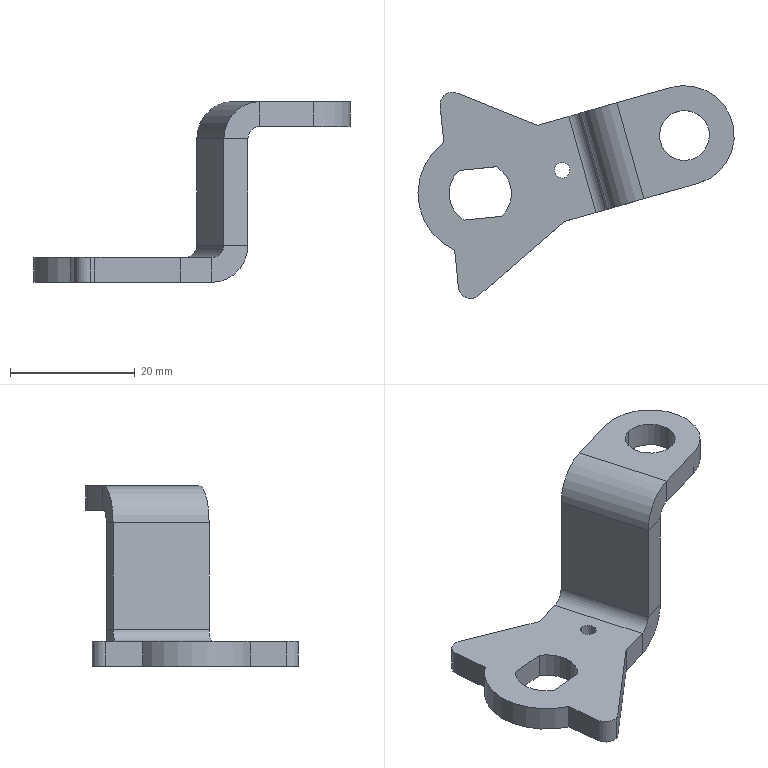Part | SolidWorks | features BaseBody 1 | 1 solid | 37 faces | box 50.722 x 34.063 x 29 mm | volume 4668 mm3 | plane 22 | cylinder 15 | commonest cylinder face diameters 4 x5 2.5 x2 8 x2 10 x2 12 x2 16 x1
STEP:
#1=CARTESIAN_POINT('',(438.908,43.386,86.7));
#2=VERTEX_POINT('',#1);
#3=CARTESIAN_POINT('',(436.735,51.085,86.7));
#4=VERTEX_POINT('',#3);
#5=CARTESIAN_POINT('',(437.822,47.235,86.7));
#6=DIRECTION('',(0.,0.,1.));
#7=DIRECTION('',(-0.2716,0.9624,0.));
#8=AXIS2_PLACEMENT_3D('',#5,#6,#7);
#9=CIRCLE('',#8,4.);
#10=EDGE_CURVE('',#2,#4,#9,.T.);
#11=ORIENTED_EDGE('',*,*,#10,.T.);
#12=CARTESIAN_POINT('',(436.735,51.085,82.7));
#13=VERTEX_POINT('',#12);
#14=CARTESIAN_POINT('',(436.735,51.085,86.7));
#15=DIRECTION('',(0.,0.,-1.));
#16=VECTOR('',#15,1000.);
#17=LINE('',#14,#16);
#18=EDGE_CURVE('',#4,#13,#17,.T.);
#19=ORIENTED_EDGE('',*,*,#18,.T.);
#20=CARTESIAN_POINT('',(438.908,43.386,82.7));
#21=VERTEX_POINT('',#20);
#22=CARTESIAN_POINT('',(437.822,47.235,82.7));
#23=DIRECTION('',(0.,0.,1.));
#24=DIRECTION('',(-0.2716,0.9624,0.));
#25=AXIS2_PLACEMENT_3D('',#22,#23,#24);
#26=CIRCLE('',#25,4.);
#27=EDGE_CURVE('',#21,#13,#26,.T.);
#28=ORIENTED_EDGE('',*,*,#27,.F.);
#29=CARTESIAN_POINT('',(438.908,43.386,86.7));
#30=DIRECTION('',(0.,0.,-1.));
#31=VECTOR('',#30,1000.);
#32=LINE('',#29,#31);
#33=EDGE_CURVE('',#2,#21,#32,.T.);
#34=ORIENTED_EDGE('',*,*,#33,.F.);
#35=EDGE_LOOP('',(#11,#19,#28,#34));
#36=FACE_OUTER_BOUND('',#35,.T.);
#37=CARTESIAN_POINT('',(437.822,47.235,86.7));
#38=DIRECTION('',(0.,0.,-1.));
#39=DIRECTION('',(0.2716,-0.9624,0.));
#40=AXIS2_PLACEMENT_3D('',#37,#38,#39);
#41=CYLINDRICAL_SURFACE('',#40,4.);
#42=ADVANCED_FACE('',(#36),#41,.F.);
#43=CARTESIAN_POINT('',(404.124,21.248,61.7));
#44=VERTEX_POINT('',#43);
#45=CARTESIAN_POINT('',(404.887,21.658,61.7));
#46=VERTEX_POINT('',#45);
#47=CARTESIAN_POINT('',(403.581,23.173,61.7));
#48=DIRECTION('',(0.,0.,1.));
#49=DIRECTION('',(0.2716,-0.9624,0.));
#50=AXIS2_PLACEMENT_3D('',#47,#48,#49);
#51=CIRCLE('',#50,2.);
#52=EDGE_CURVE('',#44,#46,#51,.T.);
#53=ORIENTED_EDGE('',*,*,#52,.F.);
#54=CARTESIAN_POINT('',(404.124,21.248,57.7));
#55=VERTEX_POINT('',#54);
#56=CARTESIAN_POINT('',(404.124,21.248,61.7));
#57=DIRECTION('',(0.,0.,-1.));
#58=VECTOR('',#57,1000.);
#59=LINE('',#56,#58);
#60=EDGE_CURVE('',#44,#55,#59,.T.);
#61=ORIENTED_EDGE('',*,*,#60,.T.);
#62=CARTESIAN_POINT('',(404.887,21.658,57.7));
#63=VERTEX_POINT('',#62);
#64=CARTESIAN_POINT('',(403.581,23.173,57.7));
#65=DIRECTION('',(0.,0.,1.));
#66=DIRECTION('',(0.2716,-0.9624,0.));
#67=AXIS2_PLACEMENT_3D('',#64,#65,#66);
#68=CIRCLE('',#67,2.);
#69=EDGE_CURVE('',#55,#63,#68,.T.);
#70=ORIENTED_EDGE('',*,*,#69,.T.);
#71=CARTESIAN_POINT('',(404.887,21.658,61.7));
#72=DIRECTION('',(0.,0.,-1.));
#73=VECTOR('',#72,1000.);
#74=LINE('',#71,#73);
#75=EDGE_CURVE('',#46,#63,#74,.T.);
#76=ORIENTED_EDGE('',*,*,#75,.F.);
#77=EDGE_LOOP('',(#53,#61,#70,#76));
#78=FACE_OUTER_BOUND('',#77,.T.);
#79=CARTESIAN_POINT('',(403.581,23.173,61.7));
#80=DIRECTION('',(0.,0.,-1.));
#81=DIRECTION('',(0.2716,-0.9624,0.));
#82=AXIS2_PLACEMENT_3D('',#79,#80,#81);
#83=CYLINDRICAL_SURFACE('',#82,2.);
#84=ADVANCED_FACE('',(#78),#83,.T.);
#85=CARTESIAN_POINT('',(418.576,40.505,61.7));
#86=VERTEX_POINT('',#85);
#87=CARTESIAN_POINT('',(417.897,42.911,61.7));
#88=VERTEX_POINT('',#87);
#89=CARTESIAN_POINT('',(418.237,41.708,61.7));
#90=DIRECTION('',(0.,0.,1.));
#91=DIRECTION('',(-0.2716,0.9624,0.));
#92=AXIS2_PLACEMENT_3D('',#89,#90,#91);
#93=CIRCLE('',#92,1.25);
#94=EDGE_CURVE('',#86,#88,#93,.T.);
#95=ORIENTED_EDGE('',*,*,#94,.T.);
#96=CARTESIAN_POINT('',(417.897,42.911,57.7));
#97=VERTEX_POINT('',#96);
#98=CARTESIAN_POINT('',(417.897,42.911,61.7));
#99=DIRECTION('',(0.,0.,-1.));
#100=VECTOR('',#99,1000.);
#101=LINE('',#98,#100);
#102=EDGE_CURVE('',#88,#97,#101,.T.);
#103=ORIENTED_EDGE('',*,*,#102,.T.);
#104=CARTESIAN_POINT('',(418.576,40.505,57.7));
#105=VERTEX_POINT('',#104);
#106=CARTESIAN_POINT('',(418.237,41.708,57.7));
#107=DIRECTION('',(0.,0.,1.));
#108=DIRECTION('',(-0.2716,0.9624,0.));
#109=AXIS2_PLACEMENT_3D('',#106,#107,#108);
#110=CIRCLE('',#109,1.25);
#111=EDGE_CURVE('',#105,#97,#110,.T.);
#112=ORIENTED_EDGE('',*,*,#111,.F.);
#113=CARTESIAN_POINT('',(418.576,40.505,61.7));
#114=DIRECTION('',(0.,0.,-1.));
#115=VECTOR('',#114,1000.);
#116=LINE('',#113,#115);
#117=EDGE_CURVE('',#86,#105,#116,.T.);
#118=ORIENTED_EDGE('',*,*,#117,.F.);
#119=EDGE_LOOP('',(#95,#103,#112,#118));
#120=FACE_OUTER_BOUND('',#119,.T.);
#121=CARTESIAN_POINT('',(418.237,41.708,61.7));
#122=DIRECTION('',(0.,0.,-1.));
#123=DIRECTION('',(0.2716,-0.9624,0.));
#124=AXIS2_PLACEMENT_3D('',#121,#122,#123);
#125=CYLINDRICAL_SURFACE('',#124,1.25);
#126=ADVANCED_FACE('',(#120),#125,.F.);
#127=CARTESIAN_POINT('',(425.062,51.947,80.7));
#128=VERTEX_POINT('',#127);
#129=CARTESIAN_POINT('',(425.062,51.947,63.7));
#130=VERTEX_POINT('',#129);
#131=CARTESIAN_POINT('',(425.062,51.947,52.207));
#132=DIRECTION('',(0.,0.,-1.));
#133=VECTOR('',#132,1000.);
#134=LINE('',#131,#133);
#135=EDGE_CURVE('',#128,#130,#134,.T.);
#136=ORIENTED_EDGE('',*,*,#135,.F.);
#137=CARTESIAN_POINT('',(429.408,36.548,80.7));
#138=VERTEX_POINT('',#137);
#139=CARTESIAN_POINT('',(427.235,44.248,80.7));
#140=DIRECTION('',(0.2716,-0.9624,0.));
#141=VECTOR('',#140,1000.);
#142=LINE('',#139,#141);
#143=EDGE_CURVE('',#128,#138,#142,.T.);
#144=ORIENTED_EDGE('',*,*,#143,.T.);
#145=CARTESIAN_POINT('',(429.408,36.548,63.7));
#146=VERTEX_POINT('',#145);
#147=CARTESIAN_POINT('',(429.408,36.548,52.207));
#148=DIRECTION('',(0.,0.,1.));
#149=VECTOR('',#148,1000.);
#150=LINE('',#147,#149);
#151=EDGE_CURVE('',#146,#138,#150,.T.);
#152=ORIENTED_EDGE('',*,*,#151,.F.);
#153=CARTESIAN_POINT('',(427.235,44.248,63.7));
#154=DIRECTION('',(0.2716,-0.9624,0.));
#155=VECTOR('',#154,1000.);
#156=LINE('',#153,#155);
#157=EDGE_CURVE('',#130,#146,#156,.T.);
#158=ORIENTED_EDGE('',*,*,#157,.F.);
#159=EDGE_LOOP('',(#136,#144,#152,#158));
#160=FACE_OUTER_BOUND('',#159,.T.);
#161=CARTESIAN_POINT('',(427.235,44.248,74.417));
#162=DIRECTION('',(-0.9624,-0.2716,0.));
#163=DIRECTION('',(-0.2716,0.9624,0.));
#164=AXIS2_PLACEMENT_3D('',#161,#162,#163);
#165=PLANE('',#164);
#166=ADVANCED_FACE('',(#160),#165,.F.);
#167=CARTESIAN_POINT('',(421.213,50.86,80.7));
#168=VERTEX_POINT('',#167);
#169=CARTESIAN_POINT('',(421.213,50.86,63.7));
#170=VERTEX_POINT('',#169);
#171=CARTESIAN_POINT('',(421.213,50.86,52.207));
#172=DIRECTION('',(0.,0.,-1.));
#173=VECTOR('',#172,1000.);
#174=LINE('',#171,#173);
#175=EDGE_CURVE('',#168,#170,#174,.T.);
#176=ORIENTED_EDGE('',*,*,#175,.F.);
#177=CARTESIAN_POINT('',(421.213,50.86,80.7));
#178=DIRECTION('',(0.9624,0.2716,0.));
#179=VECTOR('',#178,1000.);
#180=LINE('',#177,#179);
#181=EDGE_CURVE('',#168,#128,#180,.T.);
#182=ORIENTED_EDGE('',*,*,#181,.T.);
#183=ORIENTED_EDGE('',*,*,#135,.T.);
#184=CARTESIAN_POINT('',(421.213,50.86,63.7));
#185=DIRECTION('',(0.9624,0.2716,0.));
#186=VECTOR('',#185,1000.);
#187=LINE('',#184,#186);
#188=EDGE_CURVE('',#170,#130,#187,.T.);
#189=ORIENTED_EDGE('',*,*,#188,.F.);
#190=EDGE_LOOP('',(#176,#182,#183,#189));
#191=FACE_OUTER_BOUND('',#190,.T.);
#192=CARTESIAN_POINT('',(421.213,50.86,52.207));
#193=DIRECTION('',(0.2716,-0.9624,0.));
#194=DIRECTION('',(0.,0.,1.));
#195=AXIS2_PLACEMENT_3D('',#192,#193,#194);
#196=PLANE('',#195);
#197=ADVANCED_FACE('',(#191),#196,.F.);
#198=ORIENTED_EDGE('',*,*,#151,.T.);
#199=CARTESIAN_POINT('',(425.559,35.462,80.7));
#200=VERTEX_POINT('',#199);
#201=CARTESIAN_POINT('',(425.559,35.462,80.7));
#202=DIRECTION('',(-0.9624,-0.2716,0.));
#203=VECTOR('',#202,1000.);
#204=LINE('',#201,#203);
#205=EDGE_CURVE('',#138,#200,#204,.T.);
#206=ORIENTED_EDGE('',*,*,#205,.T.);
#207=CARTESIAN_POINT('',(425.559,35.462,63.7));
#208=VERTEX_POINT('',#207);
#209=CARTESIAN_POINT('',(425.559,35.462,52.207));
#210=DIRECTION('',(0.,0.,1.));
#211=VECTOR('',#210,1000.);
#212=LINE('',#209,#211);
#213=EDGE_CURVE('',#208,#200,#212,.T.);
#214=ORIENTED_EDGE('',*,*,#213,.F.);
#215=CARTESIAN_POINT('',(425.559,35.462,63.7));
#216=DIRECTION('',(-0.9624,-0.2716,0.));
#217=VECTOR('',#216,1000.);
#218=LINE('',#215,#217);
#219=EDGE_CURVE('',#146,#208,#218,.T.);
#220=ORIENTED_EDGE('',*,*,#219,.F.);
#221=EDGE_LOOP('',(#198,#206,#214,#220));
#222=FACE_OUTER_BOUND('',#221,.T.);
#223=CARTESIAN_POINT('',(425.559,35.462,52.207));
#224=DIRECTION('',(-0.2716,0.9624,0.));
#225=DIRECTION('',(0.,0.,-1.));
#226=AXIS2_PLACEMENT_3D('',#223,#224,#225);
#227=PLANE('',#226);
#228=ADVANCED_FACE('',(#222),#227,.F.);
#229=CARTESIAN_POINT('',(423.386,43.161,80.7));
#230=DIRECTION('',(0.2716,-0.9624,0.));
#231=VECTOR('',#230,1000.);
#232=LINE('',#229,#231);
#233=EDGE_CURVE('',#168,#200,#232,.T.);
#234=ORIENTED_EDGE('',*,*,#233,.F.);
#235=ORIENTED_EDGE('',*,*,#175,.T.);
#236=CARTESIAN_POINT('',(423.386,43.161,63.7));
#237=DIRECTION('',(0.2716,-0.9624,0.));
#238=VECTOR('',#237,1000.);
#239=LINE('',#236,#238);
#240=EDGE_CURVE('',#170,#208,#239,.T.);
#241=ORIENTED_EDGE('',*,*,#240,.T.);
#242=ORIENTED_EDGE('',*,*,#213,.T.);
#243=EDGE_LOOP('',(#234,#235,#241,#242));
#244=FACE_OUTER_BOUND('',#243,.T.);
#245=CARTESIAN_POINT('',(423.386,43.161,74.417));
#246=DIRECTION('',(-0.9624,-0.2716,0.));
#247=DIRECTION('',(-0.2716,0.9624,0.));
#248=AXIS2_PLACEMENT_3D('',#245,#246,#247);
#249=PLANE('',#248);
#250=ADVANCED_FACE('',(#244),#249,.T.);
#251=ORIENTED_EDGE('',*,*,#102,.F.);
#252=CARTESIAN_POINT('',(418.237,41.708,61.7));
#253=DIRECTION('',(0.,0.,1.));
#254=DIRECTION('',(-0.2716,0.9624,0.));
#255=AXIS2_PLACEMENT_3D('',#252,#253,#254);
#256=CIRCLE('',#255,1.25);
#257=EDGE_CURVE('',#88,#86,#256,.T.);
#258=ORIENTED_EDGE('',*,*,#257,.T.);
#259=ORIENTED_EDGE('',*,*,#117,.T.);
#260=CARTESIAN_POINT('',(418.237,41.708,57.7));
#261=DIRECTION('',(0.,0.,1.));
#262=DIRECTION('',(-0.2716,0.9624,0.));
#263=AXIS2_PLACEMENT_3D('',#260,#261,#262);
#264=CIRCLE('',#263,1.25);
#265=EDGE_CURVE('',#97,#105,#264,.T.);
#266=ORIENTED_EDGE('',*,*,#265,.F.);
#267=EDGE_LOOP('',(#251,#258,#259,#266));
#268=FACE_OUTER_BOUND('',#267,.T.);
#269=CARTESIAN_POINT('',(418.237,41.708,61.7));
#270=DIRECTION('',(0.,0.,-1.));
#271=DIRECTION('',(0.2716,-0.9624,0.));
#272=AXIS2_PLACEMENT_3D('',#269,#270,#271);
#273=CYLINDRICAL_SURFACE('',#272,1.25);
#274=ADVANCED_FACE('',(#268),#273,.F.);
#275=CARTESIAN_POINT('',(408.486,34.321,57.7));
#276=VERTEX_POINT('',#275);
#277=CARTESIAN_POINT('',(407.683,42.281,57.7));
#278=VERTEX_POINT('',#277);
#279=CARTESIAN_POINT('',(405.1,38.,57.7));
#280=DIRECTION('',(0.,0.,1.));
#281=DIRECTION('',(-0.2716,0.9624,0.));
#282=AXIS2_PLACEMENT_3D('',#279,#280,#281);
#283=CIRCLE('',#282,5.);
#284=EDGE_CURVE('',#276,#278,#283,.T.);
#285=ORIENTED_EDGE('',*,*,#284,.F.);
#286=CARTESIAN_POINT('',(408.486,34.321,61.7));
#287=VERTEX_POINT('',#286);
#288=CARTESIAN_POINT('',(408.486,34.321,61.7));
#289=DIRECTION('',(0.,0.,-1.));
#290=VECTOR('',#289,1000.);
#291=LINE('',#288,#290);
#292=EDGE_CURVE('',#287,#276,#291,.T.);
#293=ORIENTED_EDGE('',*,*,#292,.F.);
#294=CARTESIAN_POINT('',(407.683,42.281,61.7));
#295=VERTEX_POINT('',#294);
#296=CARTESIAN_POINT('',(405.1,38.,61.7));
#297=DIRECTION('',(0.,0.,1.));
#298=DIRECTION('',(-0.2716,0.9624,0.));
#299=AXIS2_PLACEMENT_3D('',#296,#297,#298);
#300=CIRCLE('',#299,5.);
#301=EDGE_CURVE('',#287,#295,#300,.T.);
#302=ORIENTED_EDGE('',*,*,#301,.T.);
#303=CARTESIAN_POINT('',(407.683,42.281,61.7));
#304=DIRECTION('',(0.,0.,-1.));
#305=VECTOR('',#304,1000.);
#306=LINE('',#303,#305);
#307=EDGE_CURVE('',#295,#278,#306,.T.);
#308=ORIENTED_EDGE('',*,*,#307,.T.);
#309=EDGE_LOOP('',(#285,#293,#302,#308));
#310=FACE_OUTER_BOUND('',#309,.T.);
#311=CARTESIAN_POINT('',(405.1,38.,61.7));
#312=DIRECTION('',(0.,0.,-1.));
#313=DIRECTION('',(0.2716,-0.9624,0.));
#314=AXIS2_PLACEMENT_3D('',#311,#312,#313);
#315=CYLINDRICAL_SURFACE('',#314,5.);
#316=ADVANCED_FACE('',(#310),#315,.F.);
#317=CARTESIAN_POINT('',(401.714,41.679,57.7));
#318=VERTEX_POINT('',#317);
#319=CARTESIAN_POINT('',(401.714,41.679,57.7));
#320=DIRECTION('',(-0.9949,-0.1004,0.));
#321=VECTOR('',#320,1000.);
#322=LINE('',#319,#321);
#323=EDGE_CURVE('',#278,#318,#322,.T.);
#324=ORIENTED_EDGE('',*,*,#323,.F.);
#325=ORIENTED_EDGE('',*,*,#307,.F.);
#326=CARTESIAN_POINT('',(401.714,41.679,61.7));
#327=VERTEX_POINT('',#326);
#328=CARTESIAN_POINT('',(401.714,41.679,61.7));
#329=DIRECTION('',(-0.9949,-0.1004,0.));
#330=VECTOR('',#329,1000.);
#331=LINE('',#328,#330);
#332=EDGE_CURVE('',#295,#327,#331,.T.);
#333=ORIENTED_EDGE('',*,*,#332,.T.);
#334=CARTESIAN_POINT('',(401.714,41.679,61.7));
#335=DIRECTION('',(0.,0.,-1.));
#336=VECTOR('',#335,1000.);
#337=LINE('',#334,#336);
#338=EDGE_CURVE('',#327,#318,#337,.T.);
#339=ORIENTED_EDGE('',*,*,#338,.T.);
#340=EDGE_LOOP('',(#324,#325,#333,#339));
#341=FACE_OUTER_BOUND('',#340,.T.);
#342=CARTESIAN_POINT('',(401.714,41.679,61.7));
#343=DIRECTION('',(0.1004,-0.9949,0.));
#344=DIRECTION('',(0.9949,0.1004,0.));
#345=AXIS2_PLACEMENT_3D('',#342,#343,#344);
#346=PLANE('',#345);
#347=ADVANCED_FACE('',(#341),#346,.T.);
#348=CARTESIAN_POINT('',(402.517,33.719,57.7));
#349=VERTEX_POINT('',#348);
#350=CARTESIAN_POINT('',(405.1,38.,57.7));
#351=DIRECTION('',(0.,0.,1.));
#352=DIRECTION('',(-0.2716,0.9624,0.));
#353=AXIS2_PLACEMENT_3D('',#350,#351,#352);
#354=CIRCLE('',#353,5.);
#355=EDGE_CURVE('',#318,#349,#354,.T.);
#356=ORIENTED_EDGE('',*,*,#355,.F.);
#357=ORIENTED_EDGE('',*,*,#338,.F.);
#358=CARTESIAN_POINT('',(402.517,33.719,61.7));
#359=VERTEX_POINT('',#358);
#360=CARTESIAN_POINT('',(405.1,38.,61.7));
#361=DIRECTION('',(0.,0.,1.));
#362=DIRECTION('',(-0.2716,0.9624,0.));
#363=AXIS2_PLACEMENT_3D('',#360,#361,#362);
#364=CIRCLE('',#363,5.);
#365=EDGE_CURVE('',#327,#359,#364,.T.);
#366=ORIENTED_EDGE('',*,*,#365,.T.);
#367=CARTESIAN_POINT('',(402.517,33.719,61.7));
#368=DIRECTION('',(0.,0.,-1.));
#369=VECTOR('',#368,1000.);
#370=LINE('',#367,#369);
#371=EDGE_CURVE('',#359,#349,#370,.T.);
#372=ORIENTED_EDGE('',*,*,#371,.T.);
#373=EDGE_LOOP('',(#356,#357,#366,#372));
#374=FACE_OUTER_BOUND('',#373,.T.);
#375=CARTESIAN_POINT('',(405.1,38.,61.7));
#376=DIRECTION('',(0.,0.,-1.));
#377=DIRECTION('',(0.2716,-0.9624,0.));
#378=AXIS2_PLACEMENT_3D('',#375,#376,#377);
#379=CYLINDRICAL_SURFACE('',#378,5.);
#380=ADVANCED_FACE('',(#374),#379,.F.);
#381=CARTESIAN_POINT('',(402.517,33.719,57.7));
#382=DIRECTION('',(0.9949,0.1004,0.));
#383=VECTOR('',#382,1000.);
#384=LINE('',#381,#383);
#385=EDGE_CURVE('',#349,#276,#384,.T.);
#386=ORIENTED_EDGE('',*,*,#385,.F.);
#387=ORIENTED_EDGE('',*,*,#371,.F.);
#388=CARTESIAN_POINT('',(402.517,33.719,61.7));
#389=DIRECTION('',(0.9949,0.1004,0.));
#390=VECTOR('',#389,1000.);
#391=LINE('',#388,#390);
#392=EDGE_CURVE('',#359,#287,#391,.T.);
#393=ORIENTED_EDGE('',*,*,#392,.T.);
#394=ORIENTED_EDGE('',*,*,#292,.T.);
#395=EDGE_LOOP('',(#386,#387,#393,#394));
#396=FACE_OUTER_BOUND('',#395,.T.);
#397=CARTESIAN_POINT('',(402.517,33.719,61.7));
#398=DIRECTION('',(-0.1004,0.9949,0.));
#399=DIRECTION('',(-0.9949,-0.1004,0.));
#400=AXIS2_PLACEMENT_3D('',#397,#398,#399);
#401=PLANE('',#400);
#402=ADVANCED_FACE('',(#396),#401,.T.);
#403=CARTESIAN_POINT('',(418.62,33.503,57.7));
#404=VERTEX_POINT('',#403);
#405=CARTESIAN_POINT('',(418.62,33.503,57.7));
#406=DIRECTION('',(0.7572,0.6532,0.));
#407=VECTOR('',#406,1000.);
#408=LINE('',#405,#407);
#409=EDGE_CURVE('',#63,#404,#408,.T.);
#410=ORIENTED_EDGE('',*,*,#409,.T.);
#411=CARTESIAN_POINT('',(418.62,33.503,61.7));
#412=VERTEX_POINT('',#411);
#413=CARTESIAN_POINT('',(418.62,33.503,61.7));
#414=DIRECTION('',(0.,0.,-1.));
#415=VECTOR('',#414,1000.);
#416=LINE('',#413,#415);
#417=EDGE_CURVE('',#412,#404,#416,.T.);
#418=ORIENTED_EDGE('',*,*,#417,.F.);
#419=CARTESIAN_POINT('',(418.62,33.503,61.7));
#420=DIRECTION('',(0.7572,0.6532,0.));
#421=VECTOR('',#420,1000.);
#422=LINE('',#419,#421);
#423=EDGE_CURVE('',#46,#412,#422,.T.);
#424=ORIENTED_EDGE('',*,*,#423,.F.);
#425=ORIENTED_EDGE('',*,*,#75,.T.);
#426=EDGE_LOOP('',(#410,#418,#424,#425));
#427=FACE_OUTER_BOUND('',#426,.T.);
#428=CARTESIAN_POINT('',(418.62,33.503,61.7));
#429=DIRECTION('',(-0.6532,0.7572,0.));
#430=DIRECTION('',(-0.7572,-0.6532,0.));
#431=AXIS2_PLACEMENT_3D('',#428,#429,#430);
#432=PLANE('',#431);
#433=ADVANCED_FACE('',(#427),#432,.F.);
#434=ORIENTED_EDGE('',*,*,#60,.F.);
#435=CARTESIAN_POINT('',(401.591,22.972,61.7));
#436=VERTEX_POINT('',#435);
#437=CARTESIAN_POINT('',(403.581,23.173,61.7));
#438=DIRECTION('',(0.,0.,1.));
#439=DIRECTION('',(0.2716,-0.9624,0.));
#440=AXIS2_PLACEMENT_3D('',#437,#438,#439);
#441=CIRCLE('',#440,2.);
#442=EDGE_CURVE('',#436,#44,#441,.T.);
#443=ORIENTED_EDGE('',*,*,#442,.F.);
#444=CARTESIAN_POINT('',(401.591,22.972,57.7));
#445=VERTEX_POINT('',#444);
#446=CARTESIAN_POINT('',(401.591,22.972,61.7));
#447=DIRECTION('',(0.,0.,-1.));
#448=VECTOR('',#447,1000.);
#449=LINE('',#446,#448);
#450=EDGE_CURVE('',#436,#445,#449,.T.);
#451=ORIENTED_EDGE('',*,*,#450,.T.);
#452=CARTESIAN_POINT('',(403.581,23.173,57.7));
#453=DIRECTION('',(0.,0.,1.));
#454=DIRECTION('',(0.2716,-0.9624,0.));
#455=AXIS2_PLACEMENT_3D('',#452,#453,#454);
#456=CIRCLE('',#455,2.);
#457=EDGE_CURVE('',#445,#55,#456,.T.);
#458=ORIENTED_EDGE('',*,*,#457,.T.);
#459=EDGE_LOOP('',(#434,#443,#451,#458));
#460=FACE_OUTER_BOUND('',#459,.T.);
#461=CARTESIAN_POINT('',(403.581,23.173,61.7));
#462=DIRECTION('',(0.,0.,-1.));
#463=DIRECTION('',(0.2716,-0.9624,0.));
#464=AXIS2_PLACEMENT_3D('',#461,#462,#463);
#465=CYLINDRICAL_SURFACE('',#464,2.);
#466=ADVANCED_FACE('',(#460),#465,.T.);
#467=CARTESIAN_POINT('',(400.995,28.882,57.7));
#468=VERTEX_POINT('',#467);
#469=CARTESIAN_POINT('',(401.591,22.972,57.7));
#470=DIRECTION('',(0.1004,-0.9949,0.));
#471=VECTOR('',#470,1000.);
#472=LINE('',#469,#471);
#473=EDGE_CURVE('',#468,#445,#472,.T.);
#474=ORIENTED_EDGE('',*,*,#473,.T.);
#475=ORIENTED_EDGE('',*,*,#450,.F.);
#476=CARTESIAN_POINT('',(400.995,28.882,61.7));
#477=VERTEX_POINT('',#476);
#478=CARTESIAN_POINT('',(401.591,22.972,61.7));
#479=DIRECTION('',(0.1004,-0.9949,0.));
#480=VECTOR('',#479,1000.);
#481=LINE('',#478,#480);
#482=EDGE_CURVE('',#477,#436,#481,.T.);
#483=ORIENTED_EDGE('',*,*,#482,.F.);
#484=CARTESIAN_POINT('',(400.995,28.882,61.7));
#485=DIRECTION('',(0.,0.,-1.));
#486=VECTOR('',#485,1000.);
#487=LINE('',#484,#486);
#488=EDGE_CURVE('',#477,#468,#487,.T.);
#489=ORIENTED_EDGE('',*,*,#488,.T.);
#490=EDGE_LOOP('',(#474,#475,#483,#489));
#491=FACE_OUTER_BOUND('',#490,.T.);
#492=CARTESIAN_POINT('',(401.591,22.972,61.7));
#493=DIRECTION('',(0.9949,0.1004,0.));
#494=DIRECTION('',(-0.1004,0.9949,0.));
#495=AXIS2_PLACEMENT_3D('',#492,#493,#494);
#496=PLANE('',#495);
#497=ADVANCED_FACE('',(#491),#496,.F.);
#498=CARTESIAN_POINT('',(399.256,46.115,57.7));
#499=VERTEX_POINT('',#498);
#500=CARTESIAN_POINT('',(405.1,38.,57.7));
#501=DIRECTION('',(0.,0.,1.));
#502=DIRECTION('',(-0.2716,0.9624,0.));
#503=AXIS2_PLACEMENT_3D('',#500,#501,#502);
#504=CIRCLE('',#503,10.);
#505=EDGE_CURVE('',#499,#468,#504,.T.);
#506=ORIENTED_EDGE('',*,*,#505,.T.);
#507=ORIENTED_EDGE('',*,*,#488,.F.);
#508=CARTESIAN_POINT('',(399.256,46.115,61.7));
#509=VERTEX_POINT('',#508);
#510=CARTESIAN_POINT('',(405.1,38.,61.7));
#511=DIRECTION('',(0.,0.,1.));
#512=DIRECTION('',(-0.2716,0.9624,0.));
#513=AXIS2_PLACEMENT_3D('',#510,#511,#512);
#514=CIRCLE('',#513,10.);
#515=EDGE_CURVE('',#509,#477,#514,.T.);
#516=ORIENTED_EDGE('',*,*,#515,.F.);
#517=CARTESIAN_POINT('',(399.256,46.115,61.7));
#518=DIRECTION('',(0.,0.,-1.));
#519=VECTOR('',#518,1000.);
#520=LINE('',#517,#519);
#521=EDGE_CURVE('',#509,#499,#520,.T.);
#522=ORIENTED_EDGE('',*,*,#521,.T.);
#523=EDGE_LOOP('',(#506,#507,#516,#522));
#524=FACE_OUTER_BOUND('',#523,.T.);
#525=CARTESIAN_POINT('',(405.1,38.,61.7));
#526=DIRECTION('',(0.,0.,-1.));
#527=DIRECTION('',(0.2716,-0.9624,0.));
#528=AXIS2_PLACEMENT_3D('',#525,#526,#527);
#529=CYLINDRICAL_SURFACE('',#528,10.);
#530=ADVANCED_FACE('',(#524),#529,.T.);
#531=CARTESIAN_POINT('',(398.66,52.024,57.7));
#532=VERTEX_POINT('',#531);
#533=CARTESIAN_POINT('',(399.256,46.115,57.7));
#534=DIRECTION('',(0.1004,-0.9949,0.));
#535=VECTOR('',#534,1000.);
#536=LINE('',#533,#535);
#537=EDGE_CURVE('',#532,#499,#536,.T.);
#538=ORIENTED_EDGE('',*,*,#537,.T.);
#539=ORIENTED_EDGE('',*,*,#521,.F.);
#540=CARTESIAN_POINT('',(398.66,52.024,61.7));
#541=VERTEX_POINT('',#540);
#542=CARTESIAN_POINT('',(399.256,46.115,61.7));
#543=DIRECTION('',(0.1004,-0.9949,0.));
#544=VECTOR('',#543,1000.);
#545=LINE('',#542,#544);
#546=EDGE_CURVE('',#541,#509,#545,.T.);
#547=ORIENTED_EDGE('',*,*,#546,.F.);
#548=CARTESIAN_POINT('',(398.66,52.024,61.7));
#549=DIRECTION('',(0.,0.,-1.));
#550=VECTOR('',#549,1000.);
#551=LINE('',#548,#550);
#552=EDGE_CURVE('',#541,#532,#551,.T.);
#553=ORIENTED_EDGE('',*,*,#552,.T.);
#554=EDGE_LOOP('',(#538,#539,#547,#553));
#555=FACE_OUTER_BOUND('',#554,.T.);
#556=CARTESIAN_POINT('',(399.256,46.115,61.7));
#557=DIRECTION('',(0.9949,0.1004,0.));
#558=DIRECTION('',(-0.1004,0.9949,0.));
#559=AXIS2_PLACEMENT_3D('',#556,#557,#558);
#560=PLANE('',#559);
#561=ADVANCED_FACE('',(#555),#560,.F.);
#562=CARTESIAN_POINT('',(401.396,54.081,57.7));
#563=VERTEX_POINT('',#562);
#564=CARTESIAN_POINT('',(400.65,52.225,57.7));
#565=DIRECTION('',(0.,0.,1.));
#566=DIRECTION('',(-0.2716,0.9624,0.));
#567=AXIS2_PLACEMENT_3D('',#564,#565,#566);
#568=CIRCLE('',#567,2.);
#569=EDGE_CURVE('',#563,#532,#568,.T.);
#570=ORIENTED_EDGE('',*,*,#569,.T.);
#571=ORIENTED_EDGE('',*,*,#552,.F.);
#572=CARTESIAN_POINT('',(401.396,54.081,61.7));
#573=VERTEX_POINT('',#572);
#574=CARTESIAN_POINT('',(400.65,52.225,61.7));
#575=DIRECTION('',(0.,0.,1.));
#576=DIRECTION('',(-0.2716,0.9624,0.));
#577=AXIS2_PLACEMENT_3D('',#574,#575,#576);
#578=CIRCLE('',#577,2.);
#579=EDGE_CURVE('',#573,#541,#578,.T.);
#580=ORIENTED_EDGE('',*,*,#579,.F.);
#581=CARTESIAN_POINT('',(401.396,54.081,61.7));
#582=DIRECTION('',(0.,0.,-1.));
#583=VECTOR('',#582,1000.);
#584=LINE('',#581,#583);
#585=EDGE_CURVE('',#573,#563,#584,.T.);
#586=ORIENTED_EDGE('',*,*,#585,.T.);
#587=EDGE_LOOP('',(#570,#571,#580,#586));
#588=FACE_OUTER_BOUND('',#587,.T.);
#589=CARTESIAN_POINT('',(400.65,52.225,61.7));
#590=DIRECTION('',(0.,0.,-1.));
#591=DIRECTION('',(0.2716,-0.9624,0.));
#592=AXIS2_PLACEMENT_3D('',#589,#590,#591);
#593=CYLINDRICAL_SURFACE('',#592,2.);
#594=ADVANCED_FACE('',(#588),#593,.T.);
#595=CARTESIAN_POINT('',(414.274,48.902,57.7));
#596=VERTEX_POINT('',#595);
#597=CARTESIAN_POINT('',(414.274,48.902,57.7));
#598=DIRECTION('',(-0.9278,0.3731,0.));
#599=VECTOR('',#598,1000.);
#600=LINE('',#597,#599);
#601=EDGE_CURVE('',#596,#563,#600,.T.);
#602=ORIENTED_EDGE('',*,*,#601,.T.);
#603=ORIENTED_EDGE('',*,*,#585,.F.);
#604=CARTESIAN_POINT('',(414.274,48.902,61.7));
#605=VERTEX_POINT('',#604);
#606=CARTESIAN_POINT('',(414.274,48.902,61.7));
#607=DIRECTION('',(-0.9278,0.3731,0.));
#608=VECTOR('',#607,1000.);
#609=LINE('',#606,#608);
#610=EDGE_CURVE('',#605,#573,#609,.T.);
#611=ORIENTED_EDGE('',*,*,#610,.F.);
#612=CARTESIAN_POINT('',(414.274,48.902,61.7));
#613=DIRECTION('',(0.,0.,-1.));
#614=VECTOR('',#613,1000.);
#615=LINE('',#612,#614);
#616=EDGE_CURVE('',#605,#596,#615,.T.);
#617=ORIENTED_EDGE('',*,*,#616,.T.);
#618=EDGE_LOOP('',(#602,#603,#611,#617));
#619=FACE_OUTER_BOUND('',#618,.T.);
#620=CARTESIAN_POINT('',(414.274,48.902,61.7));
#621=DIRECTION('',(-0.3731,-0.9278,0.));
#622=DIRECTION('',(0.9278,-0.3731,0.));
#623=AXIS2_PLACEMENT_3D('',#620,#621,#622);
#624=PLANE('',#623);
#625=ADVANCED_FACE('',(#619),#624,.F.);
#626=CARTESIAN_POINT('',(419.288,50.317,61.7));
#627=VERTEX_POINT('',#626);
#628=CARTESIAN_POINT('',(423.634,34.919,61.7));
#629=VERTEX_POINT('',#628);
#630=CARTESIAN_POINT('',(421.461,42.618,61.7));
#631=DIRECTION('',(0.2716,-0.9624,0.));
#632=VECTOR('',#631,1000.);
#633=LINE('',#630,#632);
#634=EDGE_CURVE('',#627,#629,#633,.T.);
#635=ORIENTED_EDGE('',*,*,#634,.F.);
#636=CARTESIAN_POINT('',(414.274,48.902,61.7));
#637=DIRECTION('',(-0.9624,-0.2716,0.));
#638=VECTOR('',#637,1000.);
#639=LINE('',#636,#638);
#640=EDGE_CURVE('',#627,#605,#639,.T.);
#641=ORIENTED_EDGE('',*,*,#640,.T.);
#642=ORIENTED_EDGE('',*,*,#610,.T.);
#643=ORIENTED_EDGE('',*,*,#579,.T.);
#644=ORIENTED_EDGE('',*,*,#546,.T.);
#645=ORIENTED_EDGE('',*,*,#515,.T.);
#646=ORIENTED_EDGE('',*,*,#482,.T.);
#647=ORIENTED_EDGE('',*,*,#442,.T.);
#648=ORIENTED_EDGE('',*,*,#52,.T.);
#649=ORIENTED_EDGE('',*,*,#423,.T.);
#650=CARTESIAN_POINT('',(418.62,33.503,61.7));
#651=DIRECTION('',(0.9624,0.2716,0.));
#652=VECTOR('',#651,1000.);
#653=LINE('',#650,#652);
#654=EDGE_CURVE('',#412,#629,#653,.T.);
#655=ORIENTED_EDGE('',*,*,#654,.T.);
#656=EDGE_LOOP('',(#635,#641,#642,#643,#644,#645,#646,#647,#648,#649,#655));
#657=FACE_OUTER_BOUND('',#656,.T.);
#658=ORIENTED_EDGE('',*,*,#392,.F.);
#659=ORIENTED_EDGE('',*,*,#365,.F.);
#660=ORIENTED_EDGE('',*,*,#332,.F.);
#661=ORIENTED_EDGE('',*,*,#301,.F.);
#662=EDGE_LOOP('',(#658,#659,#660,#661));
#663=FACE_BOUND('',#662,.T.);
#664=ORIENTED_EDGE('',*,*,#94,.F.);
#665=ORIENTED_EDGE('',*,*,#257,.F.);
#666=EDGE_LOOP('',(#664,#665));
#667=FACE_BOUND('',#666,.T.);
#668=CARTESIAN_POINT('',(437.822,47.235,61.7));
#669=DIRECTION('',(0.,0.,1.));
#670=DIRECTION('',(-0.2716,0.9624,0.));
#671=AXIS2_PLACEMENT_3D('',#668,#669,#670);
#672=PLANE('',#671);
#673=ADVANCED_FACE('',(#657,#663,#667),#672,.T.);
#674=ORIENTED_EDGE('',*,*,#640,.F.);
#675=CARTESIAN_POINT('',(419.288,50.317,57.7));
#676=VERTEX_POINT('',#675);
#677=CARTESIAN_POINT('',(419.288,50.317,61.7));
#678=DIRECTION('',(0.,0.,-1.));
#679=VECTOR('',#678,1000.);
#680=LINE('',#677,#679);
#681=EDGE_CURVE('',#627,#676,#680,.T.);
#682=ORIENTED_EDGE('',*,*,#681,.T.);
#683=CARTESIAN_POINT('',(414.274,48.902,57.7));
#684=DIRECTION('',(-0.9624,-0.2716,0.));
#685=VECTOR('',#684,1000.);
#686=LINE('',#683,#685);
#687=EDGE_CURVE('',#676,#596,#686,.T.);
#688=ORIENTED_EDGE('',*,*,#687,.T.);
#689=ORIENTED_EDGE('',*,*,#616,.F.);
#690=EDGE_LOOP('',(#674,#682,#688,#689));
#691=FACE_OUTER_BOUND('',#690,.T.);
#692=CARTESIAN_POINT('',(414.274,48.902,61.7));
#693=DIRECTION('',(0.2716,-0.9624,0.));
#694=DIRECTION('',(0.9624,0.2716,0.));
#695=AXIS2_PLACEMENT_3D('',#692,#693,#694);
#696=PLANE('',#695);
#697=ADVANCED_FACE('',(#691),#696,.F.);
#698=ORIENTED_EDGE('',*,*,#111,.T.);
#699=ORIENTED_EDGE('',*,*,#265,.T.);
#700=EDGE_LOOP('',(#698,#699));
#701=FACE_BOUND('',#700,.T.);
#702=ORIENTED_EDGE('',*,*,#355,.T.);
#703=ORIENTED_EDGE('',*,*,#385,.T.);
#704=ORIENTED_EDGE('',*,*,#284,.T.);
#705=ORIENTED_EDGE('',*,*,#323,.T.);
#706=EDGE_LOOP('',(#702,#703,#704,#705));
#707=FACE_BOUND('',#706,.T.);
#708=ORIENTED_EDGE('',*,*,#687,.F.);
#709=CARTESIAN_POINT('',(423.634,34.919,57.7));
#710=VERTEX_POINT('',#709);
#711=CARTESIAN_POINT('',(421.461,42.618,57.7));
#712=DIRECTION('',(0.2716,-0.9624,0.));
#713=VECTOR('',#712,1000.);
#714=LINE('',#711,#713);
#715=EDGE_CURVE('',#676,#710,#714,.T.);
#716=ORIENTED_EDGE('',*,*,#715,.T.);
#717=CARTESIAN_POINT('',(418.62,33.503,57.7));
#718=DIRECTION('',(0.9624,0.2716,0.));
#719=VECTOR('',#718,1000.);
#720=LINE('',#717,#719);
#721=EDGE_CURVE('',#404,#710,#720,.T.);
#722=ORIENTED_EDGE('',*,*,#721,.F.);
#723=ORIENTED_EDGE('',*,*,#409,.F.);
#724=ORIENTED_EDGE('',*,*,#69,.F.);
#725=ORIENTED_EDGE('',*,*,#457,.F.);
#726=ORIENTED_EDGE('',*,*,#473,.F.);
#727=ORIENTED_EDGE('',*,*,#505,.F.);
#728=ORIENTED_EDGE('',*,*,#537,.F.);
#729=ORIENTED_EDGE('',*,*,#569,.F.);
#730=ORIENTED_EDGE('',*,*,#601,.F.);
#731=EDGE_LOOP('',(#708,#716,#722,#723,#724,#725,#726,#727,#728,#729,#730));
#732=FACE_OUTER_BOUND('',#731,.T.);
#733=CARTESIAN_POINT('',(437.822,47.235,57.7));
#734=DIRECTION('',(0.,0.,1.));
#735=DIRECTION('',(-0.2716,0.9624,0.));
#736=AXIS2_PLACEMENT_3D('',#733,#734,#735);
#737=PLANE('',#736);
#738=ADVANCED_FACE('',(#701,#707,#732),#737,.F.);
#739=ORIENTED_EDGE('',*,*,#721,.T.);
#740=CARTESIAN_POINT('',(423.634,34.919,61.7));
#741=DIRECTION('',(0.,0.,1.));
#742=VECTOR('',#741,1000.);
#743=LINE('',#740,#742);
#744=EDGE_CURVE('',#710,#629,#743,.T.);
#745=ORIENTED_EDGE('',*,*,#744,.T.);
#746=ORIENTED_EDGE('',*,*,#654,.F.);
#747=ORIENTED_EDGE('',*,*,#417,.T.);
#748=EDGE_LOOP('',(#739,#745,#746,#747));
#749=FACE_OUTER_BOUND('',#748,.T.);
#750=CARTESIAN_POINT('',(418.62,33.503,61.7));
#751=DIRECTION('',(-0.2716,0.9624,0.));
#752=DIRECTION('',(-0.9624,-0.2716,0.));
#753=AXIS2_PLACEMENT_3D('',#750,#751,#752);
#754=PLANE('',#753);
#755=ADVANCED_FACE('',(#749),#754,.F.);
#756=ORIENTED_EDGE('',*,*,#188,.T.);
#757=CARTESIAN_POINT('',(419.288,50.317,63.7));
#758=DIRECTION('',(-0.2716,0.9624,0.));
#759=DIRECTION('',(0.,0.,-1.));
#760=AXIS2_PLACEMENT_3D('',#757,#758,#759);
#761=CIRCLE('',#760,6.);
#762=EDGE_CURVE('',#130,#676,#761,.T.);
#763=ORIENTED_EDGE('',*,*,#762,.T.);
#764=ORIENTED_EDGE('',*,*,#681,.F.);
#765=CARTESIAN_POINT('',(419.288,50.317,63.7));
#766=DIRECTION('',(-0.2716,0.9624,0.));
#767=DIRECTION('',(0.,0.,-1.));
#768=AXIS2_PLACEMENT_3D('',#765,#766,#767);
#769=CIRCLE('',#768,2.);
#770=EDGE_CURVE('',#170,#627,#769,.T.);
#771=ORIENTED_EDGE('',*,*,#770,.F.);
#772=EDGE_LOOP('',(#756,#763,#764,#771));
#773=FACE_OUTER_BOUND('',#772,.T.);
#774=CARTESIAN_POINT('',(419.288,50.317,63.7));
#775=DIRECTION('',(0.2716,-0.9624,0.));
#776=DIRECTION('',(0.,0.,1.));
#777=AXIS2_PLACEMENT_3D('',#774,#775,#776);
#778=PLANE('',#777);
#779=ADVANCED_FACE('',(#773),#778,.F.);
#780=ORIENTED_EDGE('',*,*,#634,.T.);
#781=CARTESIAN_POINT('',(423.634,34.919,63.7));
#782=DIRECTION('',(0.2716,-0.9624,0.));
#783=DIRECTION('',(0.,0.,1.));
#784=AXIS2_PLACEMENT_3D('',#781,#782,#783);
#785=CIRCLE('',#784,2.);
#786=EDGE_CURVE('',#629,#208,#785,.T.);
#787=ORIENTED_EDGE('',*,*,#786,.T.);
#788=ORIENTED_EDGE('',*,*,#240,.F.);
#789=ORIENTED_EDGE('',*,*,#770,.T.);
#790=EDGE_LOOP('',(#780,#787,#788,#789));
#791=FACE_OUTER_BOUND('',#790,.T.);
#792=CARTESIAN_POINT('',(426.255,25.633,63.7));
#793=DIRECTION('',(-0.2716,0.9624,0.));
#794=DIRECTION('',(0.,0.,-1.));
#795=AXIS2_PLACEMENT_3D('',#792,#793,#794);
#796=CYLINDRICAL_SURFACE('',#795,2.);
#797=ADVANCED_FACE('',(#791),#796,.F.);
#798=CARTESIAN_POINT('',(423.634,34.919,63.7));
#799=DIRECTION('',(0.2716,-0.9624,0.));
#800=DIRECTION('',(0.,0.,-1.));
#801=AXIS2_PLACEMENT_3D('',#798,#799,#800);
#802=CIRCLE('',#801,6.);
#803=EDGE_CURVE('',#710,#146,#802,.T.);
#804=ORIENTED_EDGE('',*,*,#803,.T.);
#805=ORIENTED_EDGE('',*,*,#219,.T.);
#806=ORIENTED_EDGE('',*,*,#786,.F.);
#807=ORIENTED_EDGE('',*,*,#744,.F.);
#808=EDGE_LOOP('',(#804,#805,#806,#807));
#809=FACE_OUTER_BOUND('',#808,.T.);
#810=CARTESIAN_POINT('',(423.634,34.919,63.7));
#811=DIRECTION('',(-0.2716,0.9624,0.));
#812=DIRECTION('',(0.,0.,-1.));
#813=AXIS2_PLACEMENT_3D('',#810,#811,#812);
#814=PLANE('',#813);
#815=ADVANCED_FACE('',(#809),#814,.F.);
#816=ORIENTED_EDGE('',*,*,#715,.F.);
#817=ORIENTED_EDGE('',*,*,#762,.F.);
#818=ORIENTED_EDGE('',*,*,#157,.T.);
#819=ORIENTED_EDGE('',*,*,#803,.F.);
#820=EDGE_LOOP('',(#816,#817,#818,#819));
#821=FACE_OUTER_BOUND('',#820,.T.);
#822=CARTESIAN_POINT('',(426.255,25.633,63.7));
#823=DIRECTION('',(-0.2716,0.9624,0.));
#824=DIRECTION('',(0.,0.,-1.));
#825=AXIS2_PLACEMENT_3D('',#822,#823,#824);
#826=CYLINDRICAL_SURFACE('',#825,6.);
#827=ADVANCED_FACE('',(#821),#826,.T.);
#828=CARTESIAN_POINT('',(426.987,52.49,86.7));
#829=VERTEX_POINT('',#828);
#830=CARTESIAN_POINT('',(426.987,52.49,82.7));
#831=VERTEX_POINT('',#830);
#832=CARTESIAN_POINT('',(426.987,52.49,86.7));
#833=DIRECTION('',(0.,0.,-1.));
#834=VECTOR('',#833,1000.);
#835=LINE('',#832,#834);
#836=EDGE_CURVE('',#829,#831,#835,.T.);
#837=ORIENTED_EDGE('',*,*,#836,.T.);
#838=CARTESIAN_POINT('',(426.987,52.49,80.7));
#839=DIRECTION('',(0.2716,-0.9624,0.));
#840=DIRECTION('',(0.,0.,-1.));
#841=AXIS2_PLACEMENT_3D('',#838,#839,#840);
#842=CIRCLE('',#841,2.);
#843=EDGE_CURVE('',#831,#128,#842,.T.);
#844=ORIENTED_EDGE('',*,*,#843,.T.);
#845=ORIENTED_EDGE('',*,*,#181,.F.);
#846=CARTESIAN_POINT('',(426.987,52.49,80.7));
#847=DIRECTION('',(0.2716,-0.9624,0.));
#848=DIRECTION('',(0.,0.,1.));
#849=AXIS2_PLACEMENT_3D('',#846,#847,#848);
#850=CIRCLE('',#849,6.);
#851=EDGE_CURVE('',#829,#168,#850,.T.);
#852=ORIENTED_EDGE('',*,*,#851,.F.);
#853=EDGE_LOOP('',(#837,#844,#845,#852));
#854=FACE_OUTER_BOUND('',#853,.T.);
#855=CARTESIAN_POINT('',(426.987,52.49,80.7));
#856=DIRECTION('',(-0.2716,0.9624,0.));
#857=DIRECTION('',(0.,0.,-1.));
#858=AXIS2_PLACEMENT_3D('',#855,#856,#857);
#859=PLANE('',#858);
#860=ADVANCED_FACE('',(#854),#859,.T.);
#861=ORIENTED_EDGE('',*,*,#233,.T.);
#862=CARTESIAN_POINT('',(431.333,37.092,86.7));
#863=VERTEX_POINT('',#862);
#864=CARTESIAN_POINT('',(431.333,37.092,80.7));
#865=DIRECTION('',(-0.2716,0.9624,0.));
#866=DIRECTION('',(0.,0.,-1.));
#867=AXIS2_PLACEMENT_3D('',#864,#865,#866);
#868=CIRCLE('',#867,6.);
#869=EDGE_CURVE('',#200,#863,#868,.T.);
#870=ORIENTED_EDGE('',*,*,#869,.T.);
#871=CARTESIAN_POINT('',(429.16,44.791,86.7));
#872=DIRECTION('',(0.2716,-0.9624,0.));
#873=VECTOR('',#872,1000.);
#874=LINE('',#871,#873);
#875=EDGE_CURVE('',#829,#863,#874,.T.);
#876=ORIENTED_EDGE('',*,*,#875,.F.);
#877=ORIENTED_EDGE('',*,*,#851,.T.);
#878=EDGE_LOOP('',(#861,#870,#876,#877));
#879=FACE_OUTER_BOUND('',#878,.T.);
#880=CARTESIAN_POINT('',(433.954,27.806,80.7));
#881=DIRECTION('',(-0.2716,0.9624,0.));
#882=DIRECTION('',(0.,0.,-1.));
#883=AXIS2_PLACEMENT_3D('',#880,#881,#882);
#884=CYLINDRICAL_SURFACE('',#883,6.);
#885=ADVANCED_FACE('',(#879),#884,.T.);
#886=CARTESIAN_POINT('',(431.333,37.092,82.7));
#887=VERTEX_POINT('',#886);
#888=CARTESIAN_POINT('',(431.333,37.092,80.7));
#889=DIRECTION('',(-0.2716,0.9624,0.));
#890=DIRECTION('',(0.,0.,-1.));
#891=AXIS2_PLACEMENT_3D('',#888,#889,#890);
#892=CIRCLE('',#891,2.);
#893=EDGE_CURVE('',#138,#887,#892,.T.);
#894=ORIENTED_EDGE('',*,*,#893,.T.);
#895=CARTESIAN_POINT('',(431.333,37.092,86.7));
#896=DIRECTION('',(0.,0.,1.));
#897=VECTOR('',#896,1000.);
#898=LINE('',#895,#897);
#899=EDGE_CURVE('',#887,#863,#898,.T.);
#900=ORIENTED_EDGE('',*,*,#899,.T.);
#901=ORIENTED_EDGE('',*,*,#869,.F.);
#902=ORIENTED_EDGE('',*,*,#205,.F.);
#903=EDGE_LOOP('',(#894,#900,#901,#902));
#904=FACE_OUTER_BOUND('',#903,.T.);
#905=CARTESIAN_POINT('',(431.333,37.092,80.7));
#906=DIRECTION('',(0.2716,-0.9624,0.));
#907=DIRECTION('',(0.,0.,1.));
#908=AXIS2_PLACEMENT_3D('',#905,#906,#907);
#909=PLANE('',#908);
#910=ADVANCED_FACE('',(#904),#909,.T.);
#911=ORIENTED_EDGE('',*,*,#143,.F.);
#912=ORIENTED_EDGE('',*,*,#843,.F.);
#913=CARTESIAN_POINT('',(429.16,44.791,82.7));
#914=DIRECTION('',(0.2716,-0.9624,0.));
#915=VECTOR('',#914,1000.);
#916=LINE('',#913,#915);
#917=EDGE_CURVE('',#831,#887,#916,.T.);
#918=ORIENTED_EDGE('',*,*,#917,.T.);
#919=ORIENTED_EDGE('',*,*,#893,.F.);
#920=EDGE_LOOP('',(#911,#912,#918,#919));
#921=FACE_OUTER_BOUND('',#920,.T.);
#922=CARTESIAN_POINT('',(433.954,27.806,80.7));
#923=DIRECTION('',(-0.2716,0.9624,0.));
#924=DIRECTION('',(0.,0.,-1.));
#925=AXIS2_PLACEMENT_3D('',#922,#923,#924);
#926=CYLINDRICAL_SURFACE('',#925,2.);
#927=ADVANCED_FACE('',(#921),#926,.F.);
#928=CARTESIAN_POINT('',(439.995,39.536,82.7));
#929=VERTEX_POINT('',#928);
#930=CARTESIAN_POINT('',(435.649,54.935,82.7));
#931=VERTEX_POINT('',#930);
#932=CARTESIAN_POINT('',(437.822,47.235,82.7));
#933=DIRECTION('',(0.,0.,1.));
#934=DIRECTION('',(-0.2716,0.9624,0.));
#935=AXIS2_PLACEMENT_3D('',#932,#933,#934);
#936=CIRCLE('',#935,8.);
#937=EDGE_CURVE('',#929,#931,#936,.T.);
#938=ORIENTED_EDGE('',*,*,#937,.T.);
#939=CARTESIAN_POINT('',(435.649,54.935,86.7));
#940=VERTEX_POINT('',#939);
#941=CARTESIAN_POINT('',(435.649,54.935,86.7));
#942=DIRECTION('',(0.,0.,-1.));
#943=VECTOR('',#942,1000.);
#944=LINE('',#941,#943);
#945=EDGE_CURVE('',#940,#931,#944,.T.);
#946=ORIENTED_EDGE('',*,*,#945,.F.);
#947=CARTESIAN_POINT('',(439.995,39.536,86.7));
#948=VERTEX_POINT('',#947);
#949=CARTESIAN_POINT('',(437.822,47.235,86.7));
#950=DIRECTION('',(0.,0.,1.));
#951=DIRECTION('',(-0.2716,0.9624,0.));
#952=AXIS2_PLACEMENT_3D('',#949,#950,#951);
#953=CIRCLE('',#952,8.);
#954=EDGE_CURVE('',#948,#940,#953,.T.);
#955=ORIENTED_EDGE('',*,*,#954,.F.);
#956=CARTESIAN_POINT('',(439.995,39.536,86.7));
#957=DIRECTION('',(0.,0.,-1.));
#958=VECTOR('',#957,1000.);
#959=LINE('',#956,#958);
#960=EDGE_CURVE('',#948,#929,#959,.T.);
#961=ORIENTED_EDGE('',*,*,#960,.T.);
#962=EDGE_LOOP('',(#938,#946,#955,#961));
#963=FACE_OUTER_BOUND('',#962,.T.);
#964=CARTESIAN_POINT('',(437.822,47.235,86.7));
#965=DIRECTION('',(0.,0.,-1.));
#966=DIRECTION('',(0.2716,-0.9624,0.));
#967=AXIS2_PLACEMENT_3D('',#964,#965,#966);
#968=CYLINDRICAL_SURFACE('',#967,8.);
#969=ADVANCED_FACE('',(#963),#968,.T.);
#970=ORIENTED_EDGE('',*,*,#18,.F.);
#971=CARTESIAN_POINT('',(437.822,47.235,86.7));
#972=DIRECTION('',(0.,0.,1.));
#973=DIRECTION('',(-0.2716,0.9624,0.));
#974=AXIS2_PLACEMENT_3D('',#971,#972,#973);
#975=CIRCLE('',#974,4.);
#976=EDGE_CURVE('',#4,#2,#975,.T.);
#977=ORIENTED_EDGE('',*,*,#976,.T.);
#978=ORIENTED_EDGE('',*,*,#33,.T.);
#979=CARTESIAN_POINT('',(437.822,47.235,82.7));
#980=DIRECTION('',(0.,0.,1.));
#981=DIRECTION('',(-0.2716,0.9624,0.));
#982=AXIS2_PLACEMENT_3D('',#979,#980,#981);
#983=CIRCLE('',#982,4.);
#984=EDGE_CURVE('',#13,#21,#983,.T.);
#985=ORIENTED_EDGE('',*,*,#984,.F.);
#986=EDGE_LOOP('',(#970,#977,#978,#985));
#987=FACE_OUTER_BOUND('',#986,.T.);
#988=CARTESIAN_POINT('',(437.822,47.235,86.7));
#989=DIRECTION('',(0.,0.,-1.));
#990=DIRECTION('',(0.2716,-0.9624,0.));
#991=AXIS2_PLACEMENT_3D('',#988,#989,#990);
#992=CYLINDRICAL_SURFACE('',#991,4.);
#993=ADVANCED_FACE('',(#987),#992,.F.);
#994=ORIENTED_EDGE('',*,*,#10,.F.);
#995=ORIENTED_EDGE('',*,*,#976,.F.);
#996=EDGE_LOOP('',(#994,#995));
#997=FACE_BOUND('',#996,.T.);
#998=CARTESIAN_POINT('',(393.518,43.044,86.7));
#999=DIRECTION('',(-0.9624,-0.2716,0.));
#1000=VECTOR('',#999,1000.);
#1001=LINE('',#998,#1000);
#1002=EDGE_CURVE('',#940,#829,#1001,.T.);
#1003=ORIENTED_EDGE('',*,*,#1002,.T.);
#1004=ORIENTED_EDGE('',*,*,#875,.T.);
#1005=CARTESIAN_POINT('',(397.864,27.645,86.7));
#1006=DIRECTION('',(0.9624,0.2716,0.));
#1007=VECTOR('',#1006,1000.);
#1008=LINE('',#1005,#1007);
#1009=EDGE_CURVE('',#863,#948,#1008,.T.);
#1010=ORIENTED_EDGE('',*,*,#1009,.T.);
#1011=ORIENTED_EDGE('',*,*,#954,.T.);
#1012=EDGE_LOOP('',(#1003,#1004,#1010,#1011));
#1013=FACE_OUTER_BOUND('',#1012,.T.);
#1014=CARTESIAN_POINT('',(417.066,41.377,86.7));
#1015=DIRECTION('',(0.,0.,1.));
#1016=DIRECTION('',(-0.2716,0.9624,0.));
#1017=AXIS2_PLACEMENT_3D('',#1014,#1015,#1016);
#1018=PLANE('',#1017);
#1019=ADVANCED_FACE('',(#997,#1013),#1018,.T.);
#1020=ORIENTED_EDGE('',*,*,#899,.F.);
#1021=CARTESIAN_POINT('',(397.864,27.645,82.7));
#1022=DIRECTION('',(0.9624,0.2716,0.));
#1023=VECTOR('',#1022,1000.);
#1024=LINE('',#1021,#1023);
#1025=EDGE_CURVE('',#887,#929,#1024,.T.);
#1026=ORIENTED_EDGE('',*,*,#1025,.T.);
#1027=ORIENTED_EDGE('',*,*,#960,.F.);
#1028=ORIENTED_EDGE('',*,*,#1009,.F.);
#1029=EDGE_LOOP('',(#1020,#1026,#1027,#1028));
#1030=FACE_OUTER_BOUND('',#1029,.T.);
#1031=CARTESIAN_POINT('',(397.864,27.645,86.7));
#1032=DIRECTION('',(-0.2716,0.9624,0.));
#1033=DIRECTION('',(-0.9624,-0.2716,0.));
#1034=AXIS2_PLACEMENT_3D('',#1031,#1032,#1033);
#1035=PLANE('',#1034);
#1036=ADVANCED_FACE('',(#1030),#1035,.F.);
#1037=ORIENTED_EDGE('',*,*,#917,.F.);
#1038=CARTESIAN_POINT('',(393.518,43.044,82.7));
#1039=DIRECTION('',(-0.9624,-0.2716,0.));
#1040=VECTOR('',#1039,1000.);
#1041=LINE('',#1038,#1040);
#1042=EDGE_CURVE('',#931,#831,#1041,.T.);
#1043=ORIENTED_EDGE('',*,*,#1042,.F.);
#1044=ORIENTED_EDGE('',*,*,#937,.F.);
#1045=ORIENTED_EDGE('',*,*,#1025,.F.);
#1046=EDGE_LOOP('',(#1037,#1043,#1044,#1045));
#1047=FACE_OUTER_BOUND('',#1046,.T.);
#1048=ORIENTED_EDGE('',*,*,#27,.T.);
#1049=ORIENTED_EDGE('',*,*,#984,.T.);
#1050=EDGE_LOOP('',(#1048,#1049));
#1051=FACE_BOUND('',#1050,.T.);
#1052=CARTESIAN_POINT('',(417.066,41.377,82.7));
#1053=DIRECTION('',(0.,0.,1.));
#1054=DIRECTION('',(-0.2716,0.9624,0.));
#1055=AXIS2_PLACEMENT_3D('',#1052,#1053,#1054);
#1056=PLANE('',#1055);
#1057=ADVANCED_FACE('',(#1047,#1051),#1056,.F.);
#1058=ORIENTED_EDGE('',*,*,#836,.F.);
#1059=ORIENTED_EDGE('',*,*,#1002,.F.);
#1060=ORIENTED_EDGE('',*,*,#945,.T.);
#1061=ORIENTED_EDGE('',*,*,#1042,.T.);
#1062=EDGE_LOOP('',(#1058,#1059,#1060,#1061));
#1063=FACE_OUTER_BOUND('',#1062,.T.);
#1064=CARTESIAN_POINT('',(393.518,43.044,86.7));
#1065=DIRECTION('',(0.2716,-0.9624,0.));
#1066=DIRECTION('',(0.9624,0.2716,0.));
#1067=AXIS2_PLACEMENT_3D('',#1064,#1065,#1066);
#1068=PLANE('',#1067);
#1069=ADVANCED_FACE('',(#1063),#1068,.F.);
#1070=CLOSED_SHELL('',(#42,#84,#126,#166,#197,#228,#250,#274,#316,#347,#380,#402,#433,#466,#497,#530,#561,#594,#625,#673,#697,#738,#755,#779,#797,#815,#827,#860,#885,#910,#927,#969,#993,#1019,#1036,#1057,#1069));
#1071=MANIFOLD_SOLID_BREP('',#1070);
#1072=CARTESIAN_POINT('',(0.,0.,0.));
#1073=DIRECTION('',(0.,0.,1.));
#1074=DIRECTION('',(1.,0.,0.));
#1075=AXIS2_PLACEMENT_3D('',#1072,#1073,#1074);
#1076=(LENGTH_UNIT()NAMED_UNIT(*)SI_UNIT(.MILLI.,.METRE.));
#1077=UNCERTAINTY_MEASURE_WITH_UNIT(LENGTH_MEASURE(0.00001),#1076,'','');
#1078=(NAMED_UNIT(*)PLANE_ANGLE_UNIT()SI_UNIT($,.RADIAN.));
#1079=(NAMED_UNIT(*)SI_UNIT($,.STERADIAN.)SOLID_ANGLE_UNIT());
#1080=(GEOMETRIC_REPRESENTATION_CONTEXT(3)GLOBAL_UNCERTAINTY_ASSIGNED_CONTEXT((#1077))GLOBAL_UNIT_ASSIGNED_CONTEXT((#1076,#1078,#1079))REPRESENTATION_CONTEXT('',''));
#1081=ADVANCED_BREP_SHAPE_REPRESENTATION('',(#1071,#1075),#1080);